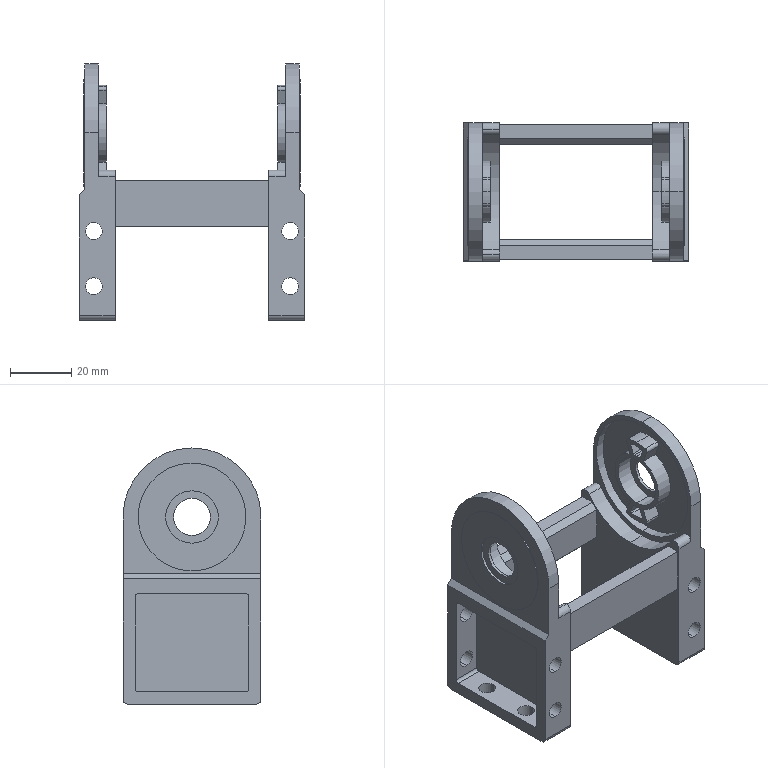Part | SolidWorks | features BaseBody 1 | 1 solid | 186 faces | box 73.47 x 44.999 x 83.497 mm | volume 38091 mm3 | cylinder 118 | plane 68 | commonest cylinder face diameters 5.5 x24 1.006 x20 20.12 x10 2 x8 2.012 x8 17.1 x8